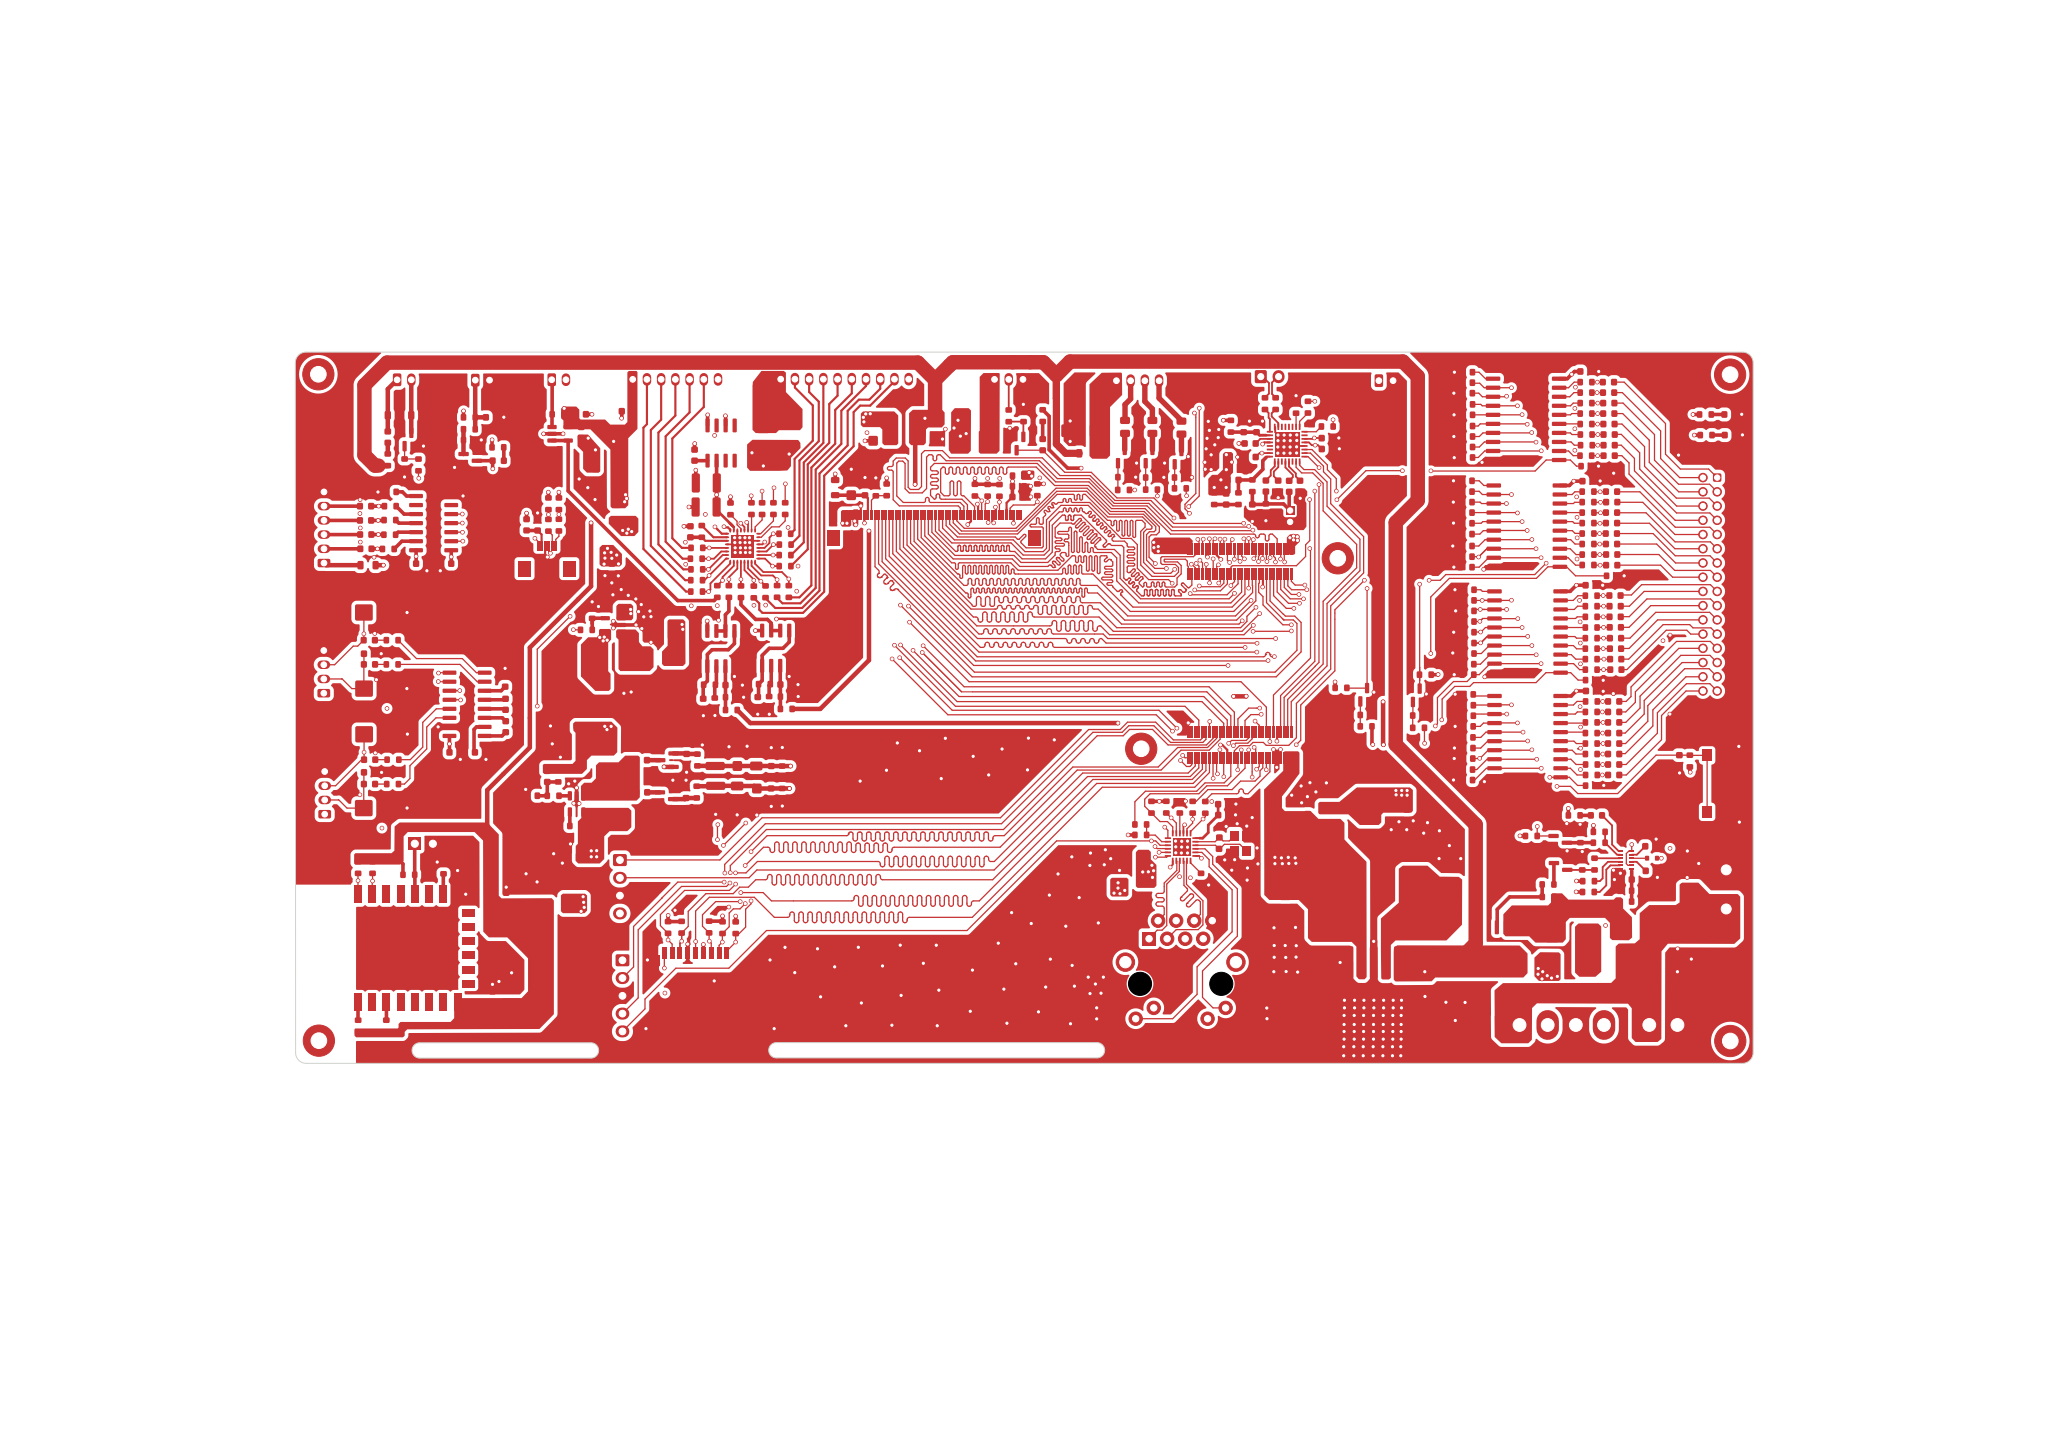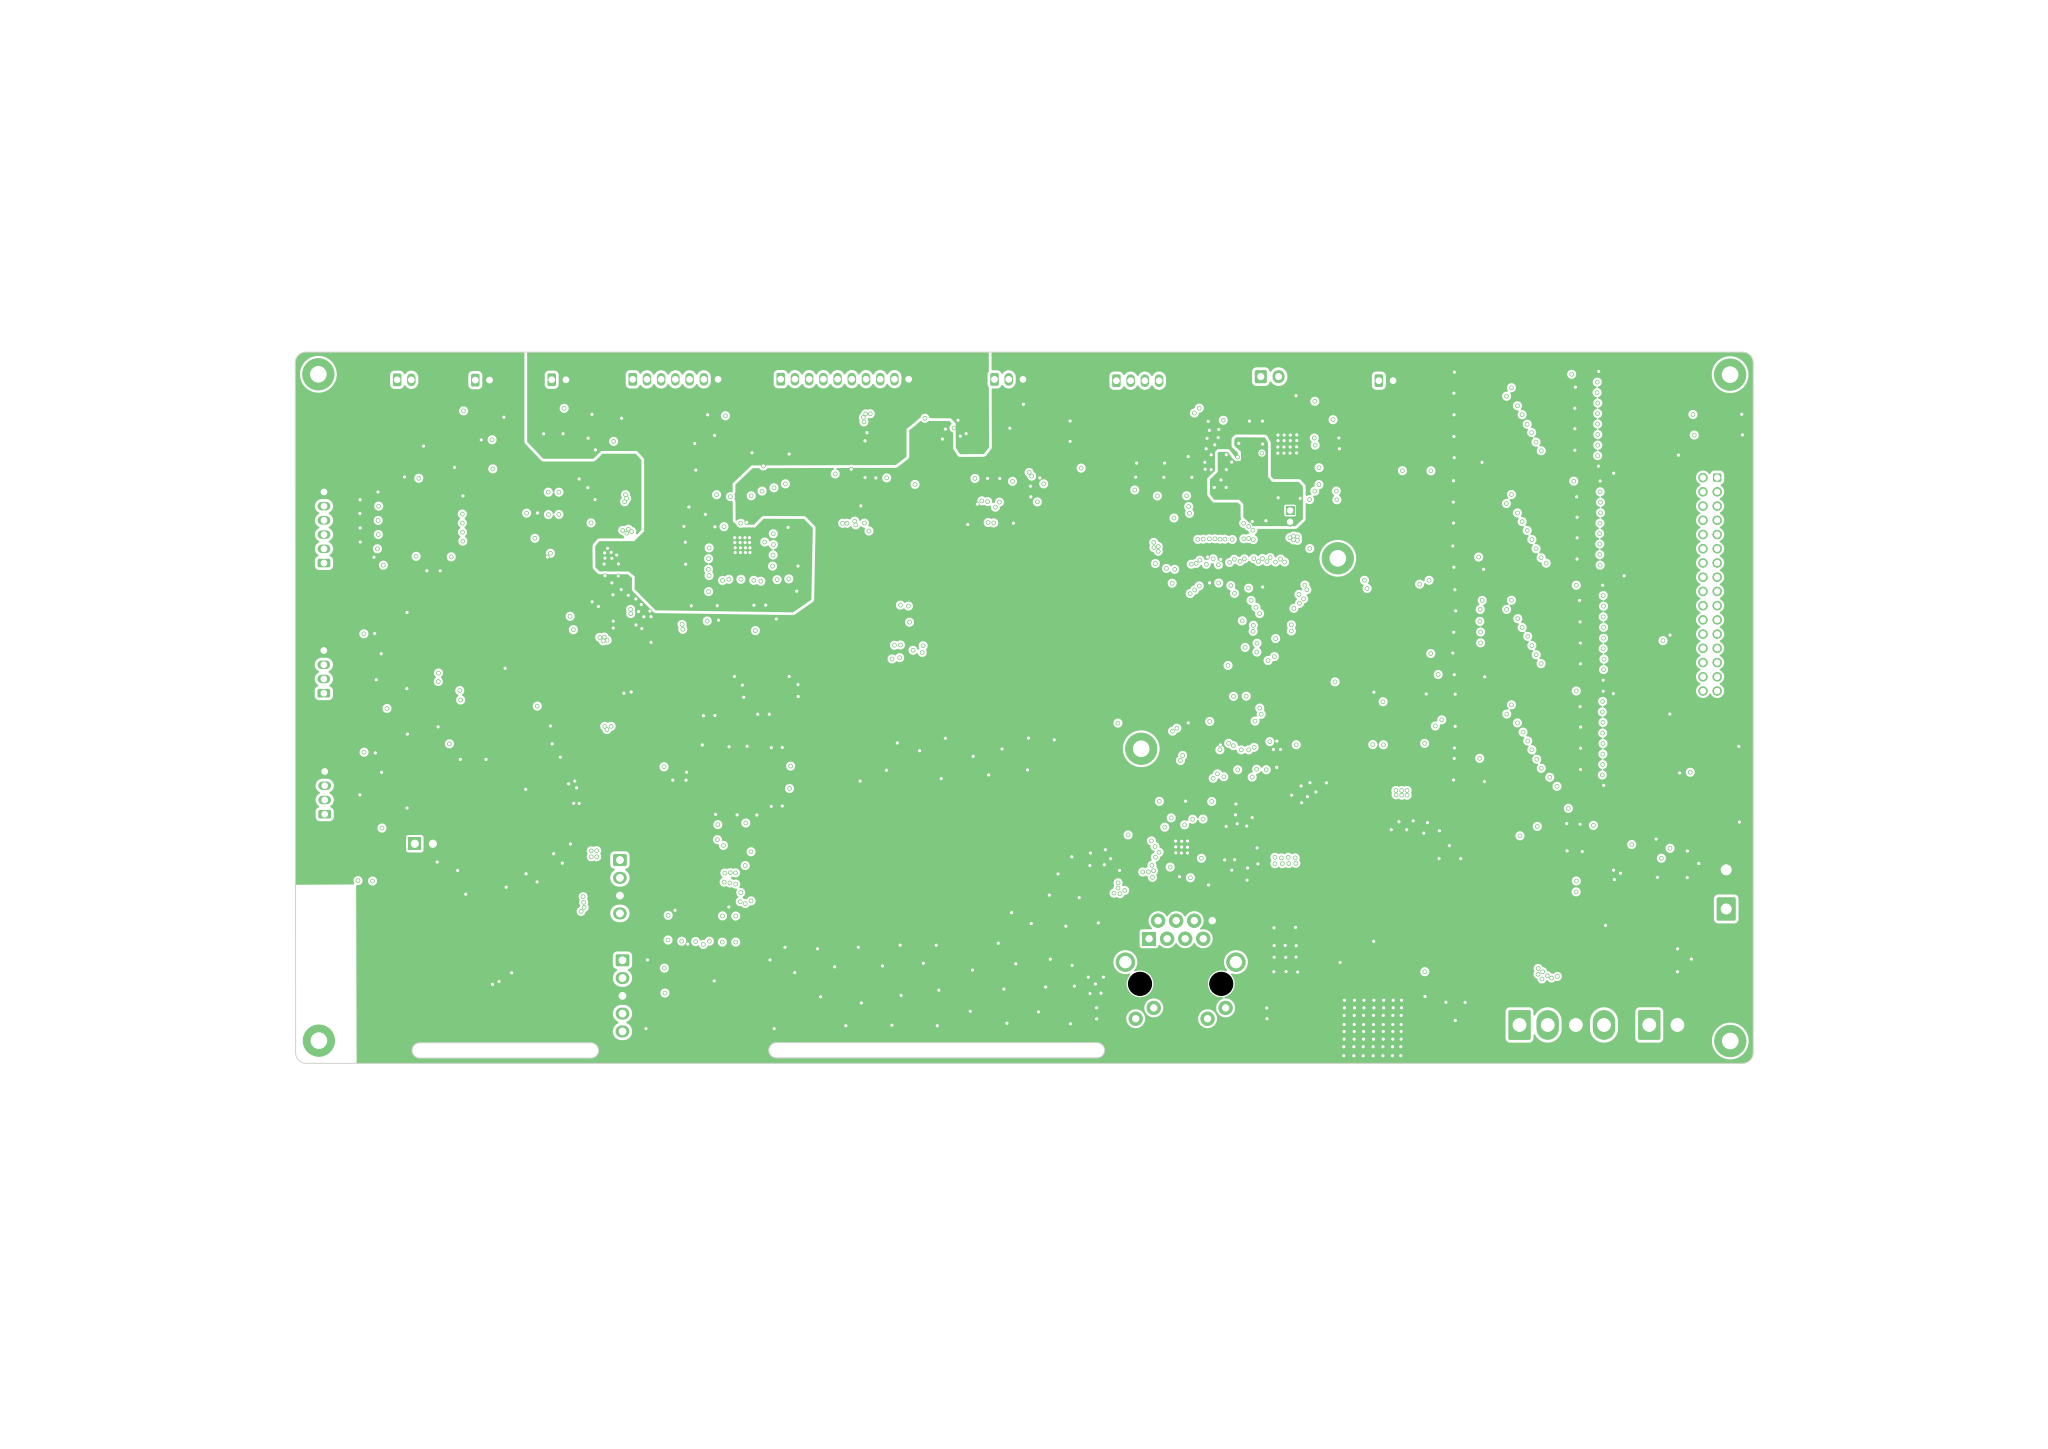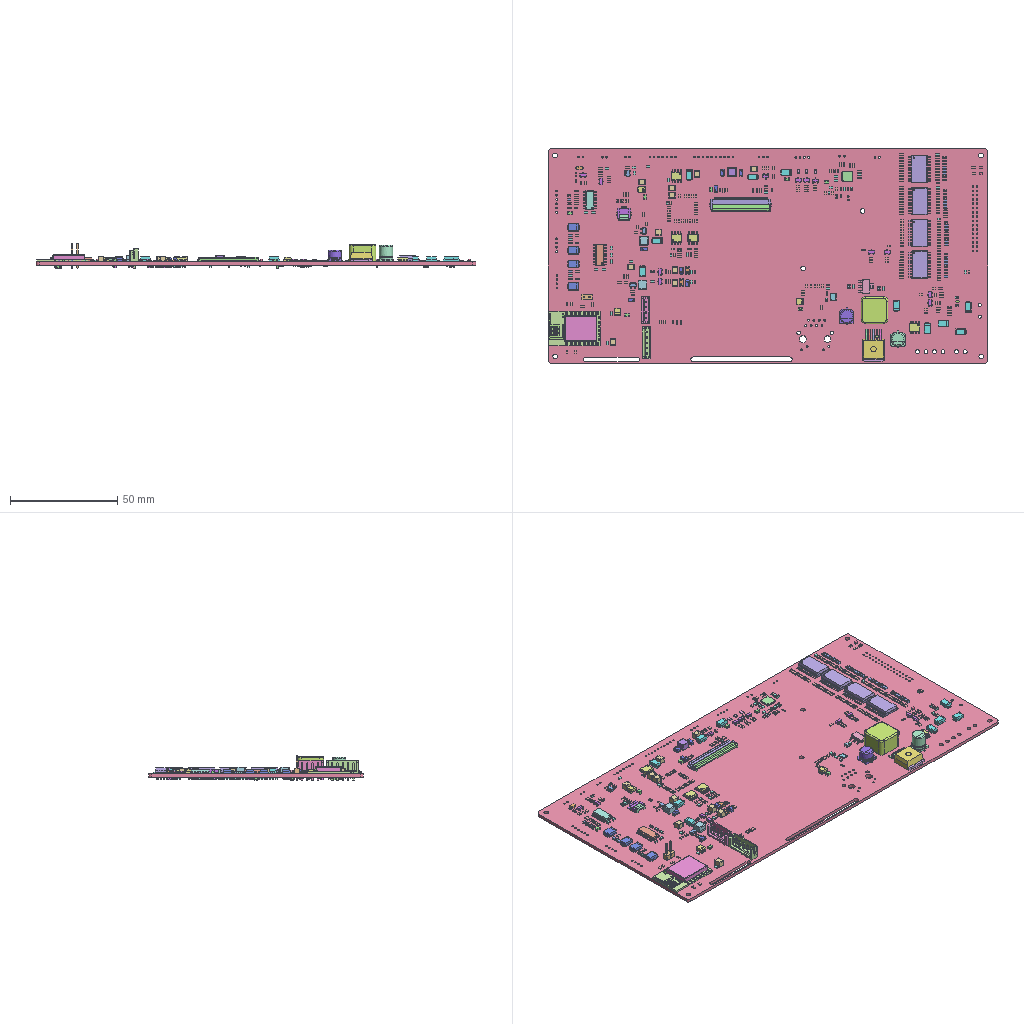Circuit board layout | KiCad | box 205.1 x 100 x 11.7 mm
Part placement, first 504 of 533 lines:
Ref,Val,Package,PosX,PosY,Rot,Side
C1,100nF,C_0603_1608Metric,108.966,-81.116,180,bottom
C2,100nF,C_0603_1608Metric,116.675,-81.04,180,bottom
C12,100nF,C_0603_1608Metric,209.093,-130.683,-90,bottom
C13,100nF,C_0603_1608Metric,140.132,-51.968,-90,bottom
C18,100nF,C_0603_1608Metric,131.521,-52.464,-90,bottom
C23,100nF/50V,C_0603_1608Metric,94.222,-55.753,180,bottom
C26,100nF/50V,C_0603_1608Metric,174.257,-117.297,-90,bottom
C29,100nF/50V,C_0603_1608Metric,174.359,-109.55,0,bottom
C33,100nF/50V,C_0603_1608Metric,176.822,-111.887,90,bottom
C34,100nF/50V,C_0603_1608Metric,174.447,-113.386,0,bottom
C48,100nF,C_0603_1608Metric,106.832,-126.035,180,bottom
C52,100nF,C_0603_1608Metric,149.273,-61.345,90,bottom
C72,1nF,C_0603_1608Metric,231.748,-56.464,180,bottom
C73,1nF,C_0603_1608Metric,231.722,-54.991,180,bottom
C74,1nF,C_0603_1608Metric,231.722,-53.492,180,bottom
C75,1nF,C_0603_1608Metric,231.773,-52.019,180,bottom
C76,1nF,C_0603_1608Metric,231.799,-50.546,180,bottom
C77,1nF,C_0603_1608Metric,231.773,-49.073,180,bottom
C78,1nF,C_0603_1608Metric,231.773,-47.6,180,bottom
C79,1nF,C_0603_1608Metric,231.773,-46.126,180,bottom
C81,1nF,C_0603_1608Metric,232.056,-71.857,180,bottom
C82,1nF,C_0603_1608Metric,232.056,-70.383,180,bottom
C83,1nF,C_0603_1608Metric,232.056,-68.885,180,bottom
C84,1nF,C_0603_1608Metric,232.056,-67.386,180,bottom
C85,1nF,C_0603_1608Metric,232.056,-65.913,180,bottom
C86,1nF,C_0603_1608Metric,232.056,-64.44,180,bottom
C87,1nF,C_0603_1608Metric,232.107,-62.967,180,bottom
C88,1nF,C_0603_1608Metric,232.054,-61.493,180,bottom
C90,1nF,C_0603_1608Metric,232.513,-86.538,180,bottom
C91,1nF,C_0603_1608Metric,232.513,-85.065,180,bottom
C92,1nF,C_0603_1608Metric,232.513,-83.591,180,bottom
C93,1nF,C_0603_1608Metric,232.488,-82.118,180,bottom
C94,1nF,C_0603_1608Metric,232.513,-80.62,180,bottom
C95,1nF,C_0603_1608Metric,232.476,-79.121,180,bottom
C96,1nF,C_0603_1608Metric,232.488,-77.622,180,bottom
C97,1nF,C_0603_1608Metric,232.488,-76.149,180,bottom
C99,1nF,C_0603_1608Metric,232.547,-101.351,180,bottom
C100,1nF,C_0603_1608Metric,232.534,-99.878,180,bottom
C101,1nF,C_0603_1608Metric,232.509,-98.405,180,bottom
C102,1nF,C_0603_1608Metric,232.509,-96.931,180,bottom
C103,1nF,C_0603_1608Metric,232.509,-95.458,180,bottom
C104,1nF,C_0603_1608Metric,232.509,-93.96,180,bottom
C105,1nF,C_0603_1608Metric,232.534,-92.486,180,bottom
C106,1nF,C_0603_1608Metric,232.534,-90.988,180,bottom
C109,270pF,C_0603_1608Metric,119.117,-67.442,0,bottom
C110,270pF,C_0603_1608Metric,119.117,-68.966,0,bottom
C111,270pF,C_0603_1608Metric,119.117,-70.439,0,bottom
C112,270pF,C_0603_1608Metric,119.117,-71.988,0,bottom
C113,270pF,C_0603_1608Metric,119.638,-75.544,-90,bottom
C114,270pF,C_0603_1608Metric,117.987,-75.544,-90,bottom
C115,270pF,C_0603_1608Metric,116.362,-75.557,-90,bottom
C116,270pF,C_0603_1608Metric,114.711,-75.557,-90,bottom
C117,270pF,C_0603_1608Metric,112.907,-75.57,-90,bottom
C118,270pF,C_0603_1608Metric,111.206,-75.557,-90,bottom
C119,270pF,C_0603_1608Metric,109.58,-75.557,-90,bottom
C120,270pF,C_0603_1608Metric,106.697,-75.57,180,bottom
C121,270pF,C_0603_1608Metric,106.697,-73.97,180,bottom
C122,270pF,C_0603_1608Metric,106.709,-72.446,180,bottom
C123,270pF,C_0603_1608Metric,106.71,-70.922,180,bottom
C124,270pF,C_0603_1608Metric,106.71,-69.423,180,bottom
C126,1uF,C_0603_1608Metric,109.957,-52.197,180,bottom
C131,100nF,C_0603_1608Metric,108.691,-63.732,180,bottom
C132,100nF,C_0603_1608Metric,115.346,-69.702,-90,bottom
C133,100nF,C_0603_1608Metric,113.64,-64.795,0,bottom
C134,100nF,C_0603_1608Metric,110.922,-68.199,-90,bottom
C139,1nF,C_0603_1608Metric,60.14,-69.555,180,bottom
C140,1nF,C_0603_1608Metric,60.127,-67.548,180,bottom
C141,1nF,C_0603_1608Metric,60.102,-65.567,180,bottom
C142,1nF,C_0603_1608Metric,60.102,-63.535,180,bottom
C145,100nF,C_0603_1608Metric,243.561,-83.337,90,bottom
C146,100nF,C_0603_1608Metric,244.336,-115.799,0,bottom
C159,330pF,C_0603_1608Metric,60.626,-82.4,0,bottom
C160,330pF,C_0603_1608Metric,60.681,-99.199,0,bottom
D9,SP0502BAHT,SOT-23,111.216,-122.633,90,bottom
D10,SP0502BAHT,SOT-23,107.452,-122.557,90,bottom
D11,SP0502BAHT,SOT-23,103.642,-122.583,90,bottom
D20,LM4040DBZ-5,SOT-23,60.325,-72.847,-90,bottom
D21,SP0502BAHT,SOT-23,106.883,-130.302,0,bottom
D30,LM4040DBZ-5,SOT-23,60.976,-88.925,0,bottom
D31,LM4040DBZ-5,SOT-23,60.272,-105.903,0,bottom
FB3,330ohm @100MHz ,L_0805_2012Metric,162.763,-128.727,-90,bottom
FB54,FerriteBead_Small,L_0805_2012Metric,61.103,-91.999,0,bottom
FB55,FerriteBead_Small,L_0805_2012Metric,60.376,-108.814,0,bottom
R31,10K,R_0603_1608Metric,164.567,-135.636,180,bottom
R32,10K,R_0603_1608Metric,185.191,-134.087,180,bottom
R33,270,R_0603_1608Metric,164.541,-134.087,0,bottom
R34,270,R_0603_1608Metric,185.217,-135.636,180,bottom
R38,33,R_0603_1608Metric,172.733,-105.88,-90,bottom
R40,10K,R_0603_1608Metric,176.441,-105.893,-90,bottom
R41,10K,R_0603_1608Metric,178.219,-105.906,-90,bottom
R45,49.9,R_0603_1608Metric,176.124,-117.297,-90,bottom
R46,49.9,R_0603_1608Metric,177.622,-117.297,-90,bottom
R47,49.9,R_0603_1608Metric,172.581,-117.323,-90,bottom
R49,49.9,R_0603_1608Metric,170.803,-117.323,-90,bottom
R76,4.7K,R_0603_1608Metric,154.582,-61.269,-90,bottom
R80,4.7K,R_0603_1608Metric,145.796,-61.316,-90,bottom
R86,4.7K,R_0603_1608Metric,147.595,-61.321,-90,bottom
R198,10K,R_0603_1608Metric,241.833,-83.287,-90,bottom
R199,10K,R_0603_1608Metric,243.586,-113.284,-90,bottom
R200,10K,R_0603_1608Metric,103.022,-131.242,0,bottom
R201,10K,R_0603_1608Metric,102.997,-129.692,180,bottom
SW1,PB_KEY,SW_Push_1P1T_NO_6x6mm_H9.5mm,239.599,-59.843,180,bottom
SW3,START,SW_Push_1P1T_NO_6x6mm_H9.5mm,239.599,-88.968,0,bottom
SW4,STOP,SW_Push_1P1T_NO_6x6mm_H9.5mm,239.599,-120.254,0,bottom
U17,LM4040DBZ-5,SOT-23,86.995,-51.562,180,bottom
C3,100nF,C_0603_1608Metric,111.506,-88.711,0,top
C4,100nF,C_0603_1608Metric,119.228,-88.635,0,top
C5,100nF,C_0603_1608Metric,107.594,-91.403,90,top
C6,100nF,C_0603_1608Metric,115.265,-91.175,90,top
C7,1uF,C_0603_1608Metric,240.878,-111.372,0,top
C8,100nF,C_0603_1608Metric,237.425,-116.046,180,top
C9,220uF/50V,CP_Elec_6.3x7.7,213.36,-130.632,-90,top
C10,10uF,C_0805_2012Metric,190.373,-106.109,90,top
C11,1uF,CP_EIA-3216-18_Kemet-A,140.208,-53.048,-90,top
C14,100nF,C_0603_1608Metric,192.608,-106.058,90,top
C15,10uF,CP_EIA-3216-18_Kemet-A,131.496,-53.023,-90,top
C16,1uF,C_0603_1608Metric,240.943,-114.827,0,top
C17,10uF/16V,C_0805_2012Metric,204.368,-106.97,-90,top
C19,100nF/16V,C_0603_1608Metric,206.553,-107.005,-90,top
C20,220uF/16V,CP_Elec_6.3x5.4,189.484,-119.996,-90,top
C21,10uF/10V,CP_EIA-3528-21_Kemet-B,93.89,-60.96,180,top
C22,10uF/10V,CP_EIA-3528-21_Kemet-B,82.675,-117.924,90,top
C24,100nF/50V,C_0603_1608Metric,79.881,-118.686,90,top
C25,100nF,C_0603_1608Metric,244.9,-99.338,-90,top
C27,22pF,C_0603_1608Metric,180.201,-109.36,90,top
C28,22pF,C_0603_1608Metric,180.15,-112.51,-90,top
C30,470pF/50V,C_0603_1608Metric,180.798,-105.461,0,top
C31,1uF/50V,C_0603_1608Metric,180.811,-106.985,0,top
C32,10uF/10V,CP_EIA-3528-21_Kemet-B,167.679,-113.139,180,top
C35,10uF/10V,C_0603_1608Metric,185.42,-52.387,90,top
C36,10uF/50V,C_0603_1608Metric,195.364,-54,0,top
C37,100nF/50V,C_0603_1608Metric,183.617,-52.387,90,top
C38,100nF/50V,C_0603_1608Metric,195.377,-55.524,0,top
C39,100nF/50V,C_0603_1608Metric,184.531,-56.654,180,top
C40,10uF/10V,C_0603_1608Metric,184.531,-54.749,180,top
C41,10uF/10V,C_0603_1608Metric,182.118,-59.88,0,top
C42,220pF/16V,C_0603_1608Metric,184.836,-64.096,90,top
C43,1uF/16V,C_0603_1608Metric,186.741,-60.731,-90,top
C44,1uF/16V,C_0603_1608Metric,188.468,-60.744,-90,top
C45,1uF/16V,C_0603_1608Metric,190.017,-60.769,-90,top
C46,1uF/16V,C_0603_1608Metric,191.541,-60.757,-90,top
C47,10uF/10V,C_0603_1608Metric,181.153,-62.56,-90,top
C49,10uF,CP_EIA-3216-18_Kemet-A,89.129,-112.446,180,top
C50,1uF,C_0603_1608Metric,89.713,-110.065,180,top
C51,10uF,CP_EIA-3216-18_Kemet-A,95.098,-88.697,0,top
C53,100nF,C_0603_1608Metric,98.908,-99.27,0,top
C54,100nF,C_0603_1608Metric,98.946,-103.787,0,top
C55,100nF,C_0603_1608Metric,85.66,-101.555,-90,top
C56,1uF,C_1210_3225Metric,101.702,-80.924,180,top
C57,100nF,C_0603_1608Metric,105.258,-99.168,-90,top
C58,10uF,C_1210_3225Metric,88.976,-96.977,180,top
C59,100nF,C_0603_1608Metric,105.181,-103.817,90,top
C60,1uF,C_0603_1608Metric,89.002,-94.456,180,top
C61,1uF,C_0603_1608Metric,151.863,-62.272,0,top
C62,10uF,CP_EIA-3216-18_Kemet-A,128.42,-60.672,90,top
C63,10uF,CP_EIA-3216-18_Kemet-A,112.395,-98.737,90,top
C64,1uF,C_1210_3225Metric,109.271,-98.61,90,top
C65,10uF,CP_EIA-3216-18_Kemet-A,115.138,-104.604,-90,top
C66,100nF/50V,C_0603_1608Metric,130.35,-61.256,90,top
C67,100nF,C_0603_1608Metric,117.17,-99.321,90,top
C68,1uF,C_1210_3225Metric,109.347,-104.35,-90,top
C69,100nF,C_0603_1608Metric,117.145,-104.02,-90,top
C70,100nF,C_0603_1608Metric,84.3,-66.209,90,top
C71,100nF,C_0603_1608Metric,231.748,-44.628,0,top
C80,100nF,C_0603_1608Metric,232.043,-60.046,0,top
C89,100nF,C_0603_1608Metric,232.486,-74.676,0,top
C98,100nF,C_0603_1608Metric,232.534,-89.54,0,top
C107,10uF,C_1210_3225Metric,119.71,-53.569,-90,top
C108,1uF,C_0603_1608Metric,96.917,-50.219,180,top
C125,270pF,C_0603_1608Metric,105.795,-67.162,90,top
C127,1uF,C_0603_1608Metric,106.381,-56.392,90,top
C128,10uF,C_1210_3225Metric,108.031,-60.303,180,top
C129,10uF,C_1210_3225Metric,108.005,-63.681,180,top
C130,10uF,C_1210_3225Metric,93.943,-57.451,180,top
C135,100nF,C_0603_1608Metric,71.378,-71.637,180,top
C136,1uF,C_0603_1608Metric,90.322,-50.648,0,top
C137,100nF,C_0603_1608Metric,67.987,-71.637,0,top
C138,1uF,C_0603_1608Metric,90.438,-53.21,-90,top
C143,100nF,C_0603_1608Metric,77.949,-132.549,90,top
C144,10uF,C_1210_3225Metric,80.645,-131.851,90,top
C153,100nF,C_0603_1608Metric,79.818,-94.564,90,top
C154,100nF,C_0603_1608Metric,77.8,-51.074,0,top
C155,100nF,C_0603_1608Metric,72.681,-98.171,0,top
C156,100nF,C_0603_1608Metric,76.262,-98.171,0,top
C157,100nF,C_0603_1608Metric,79.742,-88.163,90,top
C158,100nF,C_0603_1608Metric,79.793,-91.415,90,top
C161,330pF,C_0603_1608Metric,60.652,-84.305,0,top
C162,330pF,C_0603_1608Metric,60.655,-100.977,0,top
C163,10uF,C_1210_3225Metric,146.05,-51.486,180,top
D1,SMAJ15CA,D_SMA,242.628,-127.254,180,top
D2,SS34,D_SMA,234.544,-123.317,180,top
D3,SS34,D_SMA,227.026,-125.622,-90,top
D4,RED,LED_0603_1608Metric,252.019,-50.673,180,top
D5,RED,LED_0603_1608Metric,252.07,-53.569,180,top
D6,1N5819WT,D_SOD-523,241.056,-113.049,0,top
D7,SS34,D_SMA,212.547,-115.087,90,top
D8,RED,LED_0603_1608Metric,233.235,-107.029,180,top
D12,SS14,D_SMA,94.285,-98.965,-90,top
D13,SS14,D_SMA,101.143,-84.785,180,top
D14,BAT54S,SOT-23,102.489,-99.27,180,top
D15,BAT54S,SOT-23,102.438,-103.791,180,top
D16,ZMM16V,D_1206_3216Metric,115.062,-98.686,90,top
D17,ZMM7.5V,D_1206_3216Metric,112.37,-104.299,90,top
D18,SMAJ20A,D_SMA,246.028,-115.817,90,top
D19,SMAJ15A,D_SMA,116.053,-54.051,-90,top
D22,1N4148W,D_SOD-123,64.881,-50.78,0,top
D23,RED,LED_0603_1608Metric,63.23,-53.854,-90,top
D24,RED,LED_0603_1608Metric,78.765,-57.17,0,top
D25,SNBJ15CA,D_SMB,62.018,-78.511,180,top
D26,SMBJ15CA,D_SMB,62.052,-95.631,180,top
D27,RED,LED_0603_1608Metric,155.346,-54.915,90,top
D28,SNBJ15CA,D_SMB,62.043,-89.21,180,top
D29,SMBJ15CA,D_SMB,62.001,-106.006,180,top
D32,SMAJ15A,D_SMA,145.752,-55.066,180,top
D33,SMAJ20A,D_SMA,161.207,-52.959,180,top
F1,16V 3.5A,Fuse_1812_4532Metric,234.62,-127.635,180,top
FB1,100ohm @100MHz max. 4000mA,L_0805_2012Metric,95.402,-64.465,90,top
FB2,100ohm @100MHz max. 4000mA,L_0805_2012Metric,86.97,-119.456,180,top
FB4,330ohm @100MHz ,L_0805_2012Metric,167.94,-116.51,0,top
FB5,330ohm @100MHz ,L_0805_2012Metric,180.107,-57.389,0,top
FB6,100ohm @100MHz max. 4000mA,L_0805_2012Metric,126.159,-60.952,-90,top
FB7,100ohm @100MHz max. 4000mA,L_0603_1608Metric,82.751,-66.184,-90,top
FB8,FerriteBead_Small,L_0603_1608Metric,234.923,-46.126,0,top
FB9,FerriteBead_Small,L_0603_1608Metric,234.948,-47.6,0,top
FB10,FerriteBead_Small,L_0603_1608Metric,234.974,-49.073,0,top
FB11,FerriteBead_Small,L_0603_1608Metric,234.974,-50.546,0,top
FB12,FerriteBead_Small,L_0603_1608Metric,234.999,-52.019,0,top
FB13,FerriteBead_Small,L_0603_1608Metric,235.024,-53.492,0,top
FB14,FerriteBead_Small,L_0603_1608Metric,235.024,-54.991,0,top
FB15,FerriteBead_Small,L_0603_1608Metric,235.024,-56.464,0,top
FB16,FerriteBead_Small,L_0603_1608Metric,235.358,-61.519,0,top
FB17,FerriteBead_Small,L_0603_1608Metric,235.382,-62.992,0,top
FB18,FerriteBead_Small,L_0603_1608Metric,235.358,-64.465,0,top
FB19,FerriteBead_Small,L_0603_1608Metric,235.356,-65.938,0,top
FB20,FerriteBead_Small,L_0603_1608Metric,235.333,-67.412,0,top
FB21,FerriteBead_Small,L_0603_1608Metric,235.358,-68.885,0,top
FB22,FerriteBead_Small,L_0603_1608Metric,235.384,-70.358,0,top
FB23,FerriteBead_Small,L_0603_1608Metric,235.384,-71.857,0,top
FB24,FerriteBead_Small,L_0603_1608Metric,235.841,-76.124,0,top
FB25,FerriteBead_Small,L_0603_1608Metric,235.866,-77.622,0,top
FB26,FerriteBead_Small,L_0603_1608Metric,235.866,-79.121,0,top
FB27,FerriteBead_Small,L_0603_1608Metric,235.892,-80.594,0,top
FB28,FerriteBead_Small,L_0603_1608Metric,235.917,-82.118,0,top
FB29,FerriteBead_Small,L_0603_1608Metric,235.917,-83.591,0,top
FB30,FerriteBead_Small,L_0603_1608Metric,235.942,-85.065,0,top
FB31,FerriteBead_Small,L_0603_1608Metric,235.968,-86.538,0,top
FB32,FerriteBead_Small,L_0603_1608Metric,235.658,-91.013,0,top
FB33,FerriteBead_Small,L_0603_1608Metric,235.658,-92.486,0,top
FB34,FerriteBead_Small,L_0603_1608Metric,235.658,-93.96,0,top
FB35,FerriteBead_Small,L_0603_1608Metric,235.658,-95.458,0,top
FB36,FerriteBead_Small,L_0603_1608Metric,235.658,-96.931,0,top
FB37,FerriteBead_Small,L_0603_1608Metric,235.658,-98.405,0,top
FB38,FerriteBead_Small,L_0603_1608Metric,235.658,-99.878,0,top
FB39,FerriteBead_Small,L_0603_1608Metric,235.658,-101.351,0,top
FB40,FerriteBead_Small,L_0603_1608Metric,60.153,-69.555,180,top
FB41,FerriteBead_Small,L_0603_1608Metric,60.127,-67.548,180,top
FB42,FerriteBead_Small,L_0603_1608Metric,60.102,-65.567,180,top
FB43,FerriteBead_Small,L_0603_1608Metric,60.102,-63.56,180,top
FB44,FerriteBead_Small,L_0805_2012Metric,60.452,-71.857,0,top
FB50,FerriteBead_Small,L_0603_1608Metric,60.655,-102.628,0,top
FB51,FerriteBead_Small,L_0603_1608Metric,60.652,-85.804,0,top
FB52,FerriteBead_Small,L_0603_1608Metric,60.681,-99.199,0,top
FB53,FerriteBead_Small,L_0603_1608Metric,60.626,-82.4,0,top
FB56,FerriteBead_Small,L_0805_2012Metric,161.544,-56.134,180,top
J1,Conn_01x02,Molex_KK-396_5273-02A_1x02_P3.96mm_Vertical,240.669,-136.489,0,top
J2,Conn_01x04,Molex_KK-396_5273-04A_1x04_P3.96mm_Vertical,222.419,-136.493,0,top
J3,SWD_Debug,JST_EH_B5B-EH-A_1x05_P2.50mm_Vertical,96.241,-127.396,-90,top
J4,Conn_02x30_Counter_Clockwise,Hirose_DF12_DF12C3.0-60DS-0.5V_2x30_P0.50mm_Vertical2,183.058,-97.13,180,top
J5,Conn_01x03,JST_EH_B4B-EH-A_1x04_P2.50mm_Vertical,95.88,-113.309,-90,top
J6,Conn_02x30_Counter_Clockwise,Hirose_DF12_DF12C3.0-60DS-0.5V_2x30_P0.50mm_Vertical2,183.078,-71.315,0,top
J7,RJ45_Amphenol_RJMG1BD3B8K1ANR,RJ45_Amphenol_RJMG1BD3B8K1ANR,170.308,-124.372,0,top
J8,Conn_01x02,Molex_SPOX_5267-02A_1x02_P2.50mm_Vertical,186.024,-45.354,0,top
J9,Micro_SD_Card_Det1,TF-PUSH,111.277,-125.571,0,top
J10,Conn_01x50,Hirose_FH12-50S-0.5SH_1x50-1MP_P0.50mm_Horizontal,140.012,-66.622,0,top
J11,Conn_01x06,Hirose_FH12-6S-0.5SH_1x06-1MP_P0.50mm_Horizontal,85.612,-70.947,0,top
J12,Conn_01x02,Molex_Mini-Fit_Jr_5566-02A_2x01_P4.20mm_Vertical,251.489,-120.185,180,top
J13,Conn_02x16_Odd_Even,JST_PUD_B32B-PUDSS_2x16_P2.00mm_Vertical,250.219,-59.546,-90,top
J14,Conn_01x10,Molex_MicroClasp_55932-1030_1x10_P2.00mm_Vertical,118.495,-45.712,0,top
J15,Conn_01x07,Molex_MicroClasp_55932-0730_1x07_P2.00mm_Vertical,97.68,-45.737,0,top
J16,Conn_01x02,Molex_MicroClasp_55932-0230_1x02_P2.00mm_Vertical,86.288,-45.788,0,top
J17,Conn_01x06,Molex_MicroClasp_55932-0630_1x06_P2.00mm_Vertical,54.254,-71.557,90,top
J18,Conn_01x02,PinHeader_1x02_P2.54mm_Vertical,67.028,-111.015,90,top
J19,Conn_01x02,Molex_MicroClasp_55932-0230_1x02_P2.00mm_Vertical,202.632,-45.918,0,top
J20,Conn_01x02,Molex_MicroClasp_55932-0230_1x02_P2.00mm_Vertical,75.54,-45.847,0,top
J21,Conn_01x02,Molex_MicroClasp_55932-0230_1x02_P2.00mm_Vertical,64.541,-45.796,0,top
J22,Conn_01x04,Molex_MicroClasp_55932-0430_1x04_P2.00mm_Vertical,54.229,-89.852,90,top
J23,Conn_01x04,Molex_MicroClasp_55932-0430_1x04_P2.00mm_Vertical,54.356,-106.863,90,top
J24,Conn_01x03,Molex_MicroClasp_55932-0330_1x03_P2.00mm_Vertical,148.571,-45.739,0,top
J25,Conn_01x04,Molex_MicroClasp_55932-0430_1x04_P2.00mm_Vertical,165.716,-45.923,0,top
L1,4.7uH,L_Sunlord_SWPA4030S,135.915,-52.802,180,top
L2,33uH/3A,L_Sunlord_SWRB1207S,202.387,-117.151,180,top
L3,10uH,L_Changjiang_FNR4030S,94.285,-105.29,90,top
L4,4.7uH,L_Changjiang_FNR4030S,94.945,-84.785,0,top
MK1,Microphone,MIC-TH_BD4.5-P1.60-D0.40-L-FD,190.694,-64.973,-90,top
Q1,AO3400,SOT-23,208.371,-90.147,90,top
Q2,AO3400,SOT-23,200.975,-90.071,90,top
Q3,AO3400,SOT-23,228.194,-113.732,180,top
Q4,AO3400,SOT-23,228.142,-109.925,180,top
Q5,IRF7416,SOIC-8_3.9x4.9mm_P1.27mm,221.132,-125.247,-90,top
Q6,AO3400,SOT-23,66.542,-54.186,90,top
Q7,AO3400,SOT-23,74.826,-57.18,0,top
Q8,AO3400,SOT-23,151.679,-54.759,-90,top
Q9,AO3400,SOT-23,166.887,-56.586,90,top
Q10,AO3400,SOT-23,170.784,-56.588,90,top
Q11,AO3400,SOT-23,174.863,-56.738,90,top
R1,2K,R_0603_1608Metric,208.219,-94.719,180,top
R2,10K,R_0603_1608Metric,208.219,-92.992,180,top
R3,10K,R_0603_1608Metric,209.169,-87.249,0,top
R4,2K,R_0603_1608Metric,111.557,-92.216,0,top
R5,2K,R_0603_1608Metric,111.557,-90.413,180,top
R6,2K,R_0603_1608Metric,119.278,-92.064,0,top
R7,2K,R_0603_1608Metric,119.278,-90.337,180,top
R8,3.3K,R_0603_1608Metric,109.22,-91.353,90,top
R9,3.3K,R_0603_1608Metric,116.865,-91.149,90,top
R10,4.7K,R_0603_1608Metric,108.483,-88.66,180,top
R11,4.7K,R_0603_1608Metric,116.205,-88.584,180,top
R12,10K,R_0603_1608Metric,200.838,-94.513,180,top
R13,10K,R_0603_1608Metric,200.838,-92.913,180,top
R14,10K,R_0603_1608Metric,197.307,-89.103,180,top
R15,15K,R_0603_1608Metric,237.361,-119.145,0,top
R16,3.3K,R_0603_1608Metric,237.361,-117.621,180,top
R17,1.5K,R_0603_1608Metric,248.564,-50.673,0,top
R18,1K,R_0603_1608Metric,248.666,-53.569,0,top
R19,10K,R_0603_1608Metric,232.104,-117.799,0,top
R20,10K,R_0603_1608Metric,232.13,-116.275,0,top
R21,10K,R_0603_1608Metric,233.629,-109.347,0,top
R22,1K,R_0603_1608Metric,230.111,-107.029,0,top
R23,120,R_0603_1608Metric,232.967,-113.874,-90,top
R24,120,R_0603_1608Metric,233.629,-110.871,180,top
R25,100K,R_0603_1608Metric,226.441,-118.491,180,top
R26,10K,R_0603_1608Metric,231.24,-113.874,-90,top
R27,10K,R_0603_1608Metric,230.987,-110.038,-90,top
R28,120,R_0603_1608Metric,226.428,-116.738,0,top
R29,10K,R_0603_1608Metric,224.078,-109.925,180,top
R30,10K,R_0603_1608Metric,246.373,-99.389,90,top
R35,33,R_0603_1608Metric,176.441,-105.88,-90,top
R36,33,R_0603_1608Metric,178.219,-105.906,-90,top
R37,10K,R_0603_1608Metric,174.633,-105.868,-90,top
R39,33,R_0603_1608Metric,169.139,-108.306,0,top
R42,10K,R_0603_1608Metric,172.733,-105.867,-90,top
R43,10K,R_0603_1608Metric,170.65,-105.88,-90,top
R44,10K,R_0603_1608Metric,169.139,-109.779,0,top
R48,12.1K,R_0603_1608Metric,177.622,-116.002,-90,top
R50,0,R_0603_1608Metric,181.813,-52.324,-90,top
R51,100,R_0603_1608Metric,195.377,-52.362,180,top
R52,100,R_0603_1608Metric,192.659,-49.644,-90,top
R53,100,R_0603_1608Metric,190.983,-49.669,-90,top
R54,0,R_0603_1608Metric,186.614,-49.149,90,top
R55,0,R_0603_1608Metric,188.112,-49.149,90,top
R56,68,R_0603_1608Metric,184.836,-60.693,-90,top
R57,4.7K,R_0603_1608Metric,186.741,-64.059,-90,top
R58,68,R_0603_1608Metric,182.88,-62.508,-90,top
R59,4.7K,R_0603_1608Metric,179.476,-62.509,90,top
R60,10K,R_0603_1608Metric,112.166,-122.821,-90,top
R61,10K,R_0603_1608Metric,110.312,-122.809,-90,top
R62,10K,R_0603_1608Metric,108.428,-122.721,-90,top
R63,10K,R_0603_1608Metric,104.557,-122.748,-90,top
R64,10K,R_0603_1608Metric,102.652,-122.786,-90,top
R65,100K,R_0603_1608Metric,89.662,-108.517,0,top
R66,10K,R_0603_1608Metric,91.161,-80.95,0,top
R67,4.7K,R_0603_1608Metric,133.401,-61.265,90,top
R68,4.7K,R_0603_1608Metric,131.877,-61.282,-90,top
R69,47K,R_0603_1608Metric,91.973,-78.511,-90,top
R70,4.7K,R_0603_1608Metric,149.264,-61.346,90,top
R71,10K,R_0603_1608Metric,86.487,-104.274,180,top
R72,100K,R_0603_1608Metric,87.198,-101.498,90,top
R73,13K,R_0603_1608Metric,83.439,-104.267,0,top
R74,2,R_0603_1608Metric,96.088,-76.886,-90,top
R75,4.7K,R_0603_1608Metric,154.591,-61.26,90,top
R77,2.2K,R_0603_1608Metric,106.782,-99.245,-90,top
R78,10K,R_0603_1608Metric,118.694,-99.27,-90,top
R79,4.7K,R_0603_1608Metric,145.812,-61.307,90,top
R81,2.2K,R_0603_1608Metric,106.68,-103.754,90,top
R82,100K,R_0603_1608Metric,151.927,-59.275,0,top
R83,13K,R_0603_1608Metric,151.914,-60.774,180,top
R84,4.7K,R_0603_1608Metric,118.694,-104.071,90,top
R85,4.7K,R_0603_1608Metric,147.599,-61.328,90,top
R87,47K,R_0603_1608Metric,87.297,-63.224,90,top
R88,47K,R_0603_1608Metric,85.824,-63.224,90,top
R89,100,R_0603_1608Metric,85.824,-66.247,90,top
R90,100,R_0603_1608Metric,87.297,-66.222,90,top
R91,10K,R_0603_1608Metric,214.958,-46.203,180,top
R92,10K,R_0603_1608Metric,214.958,-47.676,180,top
R93,10K,R_0603_1608Metric,214.984,-49.251,180,top
R94,10K,R_0603_1608Metric,214.984,-50.724,180,top
R95,10K,R_0603_1608Metric,214.984,-52.299,180,top
R96,10K,R_0603_1608Metric,214.984,-53.772,180,top
R97,10K,R_0603_1608Metric,214.984,-55.245,180,top
R98,10K,R_0603_1608Metric,214.984,-56.718,180,top
R99,10K,R_0603_1608Metric,231.9,-57.937,0,top
R100,10K,R_0603_1608Metric,214.971,-44.729,180,top
R101,120,R_0603_1608Metric,231.773,-46.126,0,top
R102,120,R_0603_1608Metric,231.773,-47.6,0,top
R103,120,R_0603_1608Metric,231.773,-49.073,0,top
R104,120,R_0603_1608Metric,231.773,-50.546,0,top
R105,120,R_0603_1608Metric,231.773,-52.019,0,top
R106,120,R_0603_1608Metric,231.799,-53.492,0,top
R107,120,R_0603_1608Metric,231.824,-54.991,0,top
R108,120,R_0603_1608Metric,231.748,-56.464,0,top
R109,10K,R_0603_1608Metric,214.911,-61.519,180,top
R110,10K,R_0603_1608Metric,214.911,-62.992,180,top
R111,10K,R_0603_1608Metric,214.911,-64.465,180,top
R112,10K,R_0603_1608Metric,214.911,-65.964,180,top
R113,10K,R_0603_1608Metric,214.911,-67.488,180,top
R114,10K,R_0603_1608Metric,214.911,-69.164,180,top
R115,10K,R_0603_1608Metric,214.911,-70.663,180,top
R116,10K,R_0603_1608Metric,214.911,-72.136,180,top
R117,10K,R_0603_1608Metric,235.483,-73.355,0,top
R118,10K,R_0603_1608Metric,214.911,-59.995,180,top
R119,120,R_0603_1608Metric,232.054,-61.519,0,top
R120,120,R_0603_1608Metric,232.054,-62.992,0,top
R121,120,R_0603_1608Metric,232.056,-64.465,0,top
R122,120,R_0603_1608Metric,232.056,-65.938,0,top
R123,120,R_0603_1608Metric,232.054,-67.412,0,top
R124,120,R_0603_1608Metric,232.054,-68.885,0,top
R125,120,R_0603_1608Metric,232.056,-70.37,0,top
R126,120,R_0603_1608Metric,232.056,-71.831,0,top
R127,10K,R_0603_1608Metric,215.191,-76.81,180,top
R128,10K,R_0603_1608Metric,215.191,-78.283,180,top
R129,10K,R_0603_1608Metric,215.191,-79.781,180,top
R130,10K,R_0603_1608Metric,215.191,-81.28,180,top
R131,10K,R_0603_1608Metric,215.191,-82.804,180,top
R132,10K,R_0603_1608Metric,215.191,-84.277,180,top
R133,10K,R_0603_1608Metric,215.165,-85.776,180,top
R134,10K,R_0603_1608Metric,215.165,-87.249,180,top
R135,10K,R_0603_1608Metric,232.527,-88.011,0,top
R136,10K,R_0603_1608Metric,215.191,-75.311,180,top
R137,120,R_0603_1608Metric,232.501,-76.149,0,top
R138,120,R_0603_1608Metric,232.501,-77.622,0,top
R139,120,R_0603_1608Metric,232.501,-79.121,0,top
R140,120,R_0603_1608Metric,232.501,-80.62,0,top
R141,120,R_0603_1608Metric,232.501,-82.118,0,top
R142,120,R_0603_1608Metric,232.501,-83.591,0,top
R143,120,R_0603_1608Metric,232.501,-85.065,0,top
R144,120,R_0603_1608Metric,232.501,-86.542,0,top
R145,10K,R_0603_1608Metric,215.096,-91.547,180,top
R146,10K,R_0603_1608Metric,215.096,-93.02,180,top
R147,10K,R_0603_1608Metric,215.071,-94.518,180,top
R148,10K,R_0603_1608Metric,215.046,-96.068,180,top
R149,10K,R_0603_1608Metric,215.046,-97.566,180,top
R150,10K,R_0603_1608Metric,215.02,-99.04,180,top
R151,10K,R_0603_1608Metric,214.983,-100.589,180,top
R152,10K,R_0603_1608Metric,214.983,-102.062,180,top
R153,10K,R_0603_1608Metric,232.534,-102.85,0,top
R154,10K,R_0603_1608Metric,215.084,-90.023,180,top
R155,120,R_0603_1608Metric,232.534,-91.013,0,top
R156,120,R_0603_1608Metric,232.509,-92.486,0,top
R157,120,R_0603_1608Metric,232.509,-93.96,0,top
R158,120,R_0603_1608Metric,232.509,-95.458,0,top
R159,120,R_0603_1608Metric,232.509,-96.931,0,top
R160,120,R_0603_1608Metric,232.509,-98.405,0,top
R161,120,R_0603_1608Metric,232.534,-99.878,0,top
R162,120,R_0603_1608Metric,232.534,-101.351,0,top
R163,33,R_0603_1608Metric,119.08,-67.442,180,top
R164,33,R_0603_1608Metric,119.13,-68.966,180,top
R165,33,R_0603_1608Metric,119.105,-70.439,180,top
R166,33,R_0603_1608Metric,119.105,-71.988,180,top
R167,33,R_0603_1608Metric,119.638,-75.557,90,top
R168,33,R_0603_1608Metric,117.987,-75.544,90,top
R169,33,R_0603_1608Metric,116.362,-75.595,90,top
R170,33,R_0603_1608Metric,114.711,-75.621,90,top
R171,33,R_0603_1608Metric,112.907,-75.595,90,top
R172,33,R_0603_1608Metric,111.206,-75.557,90,top
R173,33,R_0603_1608Metric,109.58,-75.557,90,top
R174,33,R_0603_1608Metric,106.671,-75.57,0,top
R175,33,R_0603_1608Metric,106.671,-73.97,0,top
R176,33,R_0603_1608Metric,106.697,-72.446,0,top
R177,33,R_0603_1608Metric,106.62,-70.947,0,top
R178,33,R_0603_1608Metric,106.71,-69.423,0,top
R179,33,R_0603_1608Metric,107.396,-67.112,-90,top
R180,0,R_0603_1608Metric,94.742,-72.517,90,top
R181,4.7K,R_0603_1608Metric,111.434,-63.937,90,top
R182,0,R_0603_1608Metric,117.475,-63.906,90,top
R183,0,R_0603_1608Metric,115.879,-63.911,90,top
R184,0,R_0603_1608Metric,114.381,-63.911,90,top
R185,22,R_0603_1608Metric,119.126,-63.906,90,top
R186,10K,R_0603_1608Metric,63.582,-61.554,0,top
R187,10K,R_0603_1608Metric,87.173,-50.648,180,top
R188,120,R_0603_1608Metric,63.302,-69.58,180,top
R189,120,R_0603_1608Metric,63.506,-67.573,180,top
R190,120,R_0603_1608Metric,63.531,-65.516,180,top
R191,120,R_0603_1608Metric,63.582,-63.56,180,top
R192,10K,R_0603_1608Metric,59.06,-136.644,90,top
R193,10K,R_0603_1608Metric,63.022,-136.644,90,top
R194,10K,R_0603_1608Metric,71.067,-114.419,90,top
R195,10K,R_0603_1608Metric,66.19,-115.371,0,top
R196,4.7K,R_0603_1608Metric,59.053,-114.355,-90,top
R197,4.7K,R_0603_1608Metric,61.085,-114.355,-90,top
R205,4.7K,R_0603_1608Metric,74.701,-51.074,0,top
R206,220,R_0603_1608Metric,67.548,-57.765,90,top
R207,220,R_0603_1608Metric,74.701,-52.75,180,top
R208,10K,R_0603_1608Metric,65.592,-57.752,90,top
R209,10K,R_0603_1608Metric,74.701,-54.274,180,top
R210,10K,R_0603_1608Metric,63.23,-57.041,-90,top
R211,2K,R_0603_1608Metric,78.715,-55.29,180,top
R212,100,R_0603_1608Metric,63.906,-102.628,180,top
R213,100,R_0603_1608Metric,63.852,-85.804,180,top
R214,100,R_0603_1608Metric,63.957,-99.199,180,top
R215,100,R_0603_1608Metric,63.852,-82.4,180,top
R216,2K,R_0603_1608Metric,155.346,-50.838,90,top
R217,10K,R_0603_1608Metric,152.654,-50.851,-90,top
R218,220,R_0603_1608Metric,150.571,-50.862,-90,top
R219,220,R_0603_1608Metric,166.725,-61.282,0,top
Pad and via stacks:
via_type,start_layer,end_layer,diameter_mm,drill_mm,count
through,F.Cu,B.Cu,0.508,0.3048,931
Design rules, without the lines most boards share:
# KiCad design rules of  (from the KiCad project file, unit mm)
max_error = 0.005
min_clearance = 0.0
min_connection = 0.0
min_copper_edge_clearance = 0.0
min_hole_clearance = 0.25
min_hole_to_hole = 0.2032
min_microvia_diameter = 0.2
min_microvia_drill = 0.1
min_resolved_spokes = 2
min_silk_clearance = 0.0
min_text_height = 0.762
min_text_thickness = 0.08
min_through_hole_diameter = 0.3048
min_track_width = 0.0
min_via_annular_width = 0.1016
min_via_diameter = 0.508
solder_mask_clearance = 0.0
solder_mask_min_width = 0.0
solder_mask_to_copper_clearance = 0.0
use_height_for_length_calcs = True
defaults = {"board_outline_line_width": 0.1, "copper_line_width": 0.2, "copper_text_italic": false, "copper_text_size_h": 1.5, "copper_text_size_v": 1.5, "copper_text_thickness": 0.3, "copper_text_upright": false, "courtyard_line_width": 0.05, "dimension_precision": 4, "dimension_units": 3, "dimensions": {"arrow_length": 1270000, "extension_offset": 500000, "keep_text_aligned": true, "suppress_zeroes": false, "text_position": 0, "units_format": 1}, "fab_line_width": 0.1, "fab_text_italic": false, "fab_text_size_h": 1.0, "fab_text_size_v": 1.0, "fab_text_thickness": 0.15, "fab_text_upright": false, "other_line_width": 0.15, "other_text_italic": false, "other_text_size_h": 1.0, "other_text_size_v": 1.0, "other_text_thickness": 0.15, "other_text_upright": false, "pads": {"drill": 0.762, "height": 1.524, "width": 1.524}, "silk_line_width": 0.15, "silk_text_italic": false, "silk_text_size_h": 0.762, "silk_text_size_v": 0.762, "silk_text_thickness": 0.15, "silk_text_upright": false, "zones": {"min_clearance": 0.5}}
track_widths = [0.0]
via_dimensions = [{"diameter": 0.0, "drill": 0.0}]
diff_pair_dimensions = [{"gap": 0.0, "via_gap": 0.0, "width": 0.0}]
# copper zones (pour): pad connection, clearance mm, minimum width mm, count
zone connect_pads=thermal_reliefs clearance=0 min_thickness=0.254 count=1
zone connect_pads=yes clearance=0.254 min_thickness=0.25 count=9
zone connect_pads=yes clearance=0.1524 min_thickness=0.25 count=24
zone connect_pads=yes clearance=0.508 min_thickness=0.25 count=2
zone connect_pads=yes clearance=0.1524 min_thickness=0.1524 count=10
zone connect_pads=yes clearance=0.5 min_thickness=0.25 count=3
zone connect_pads=yes clearance=0.381 min_thickness=0.25 count=5
Classes set for this board:
# KiCad net classes of  (from the KiCad project file, unit mm)
{"bus_width": 12, "clearance": 0.1524, "diff_pair_gap": 0.1778, "diff_pair_via_gap": 0.25, "diff_pair_width": 0.1778, "line_style": 0, "microvia_diameter": 0.508, "microvia_drill": 0.1, "name": "Default", "pcb_color": "rgba(0, 0, 0, 0.000)", "schematic_color": "rgba(0, 0, 0, 0.000)", "track_width": 0.1778, "via_diameter": 0.508, "via_drill": 0.3048, "wire_width": 6}